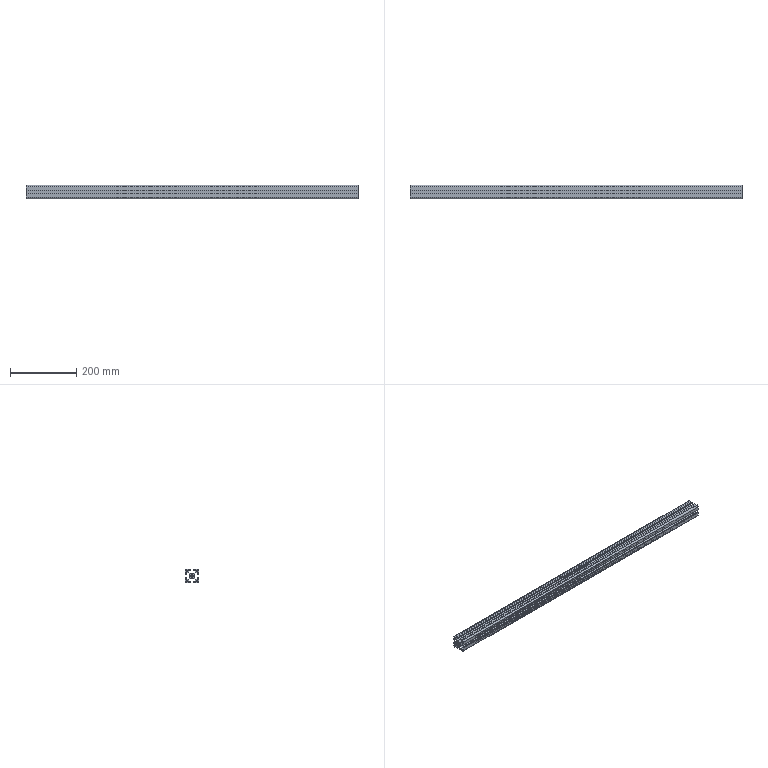Part | SolidWorks | features WeldMemberFeat 1, WeldmentFeature 1 | 1 solid | 104 faces | box 1000 x 40 x 40 mm | volume 576545 mm3 | plane 94 | cylinder 10 | commonest cylinder face diameters 5 x4 9 x4 6.8 x2